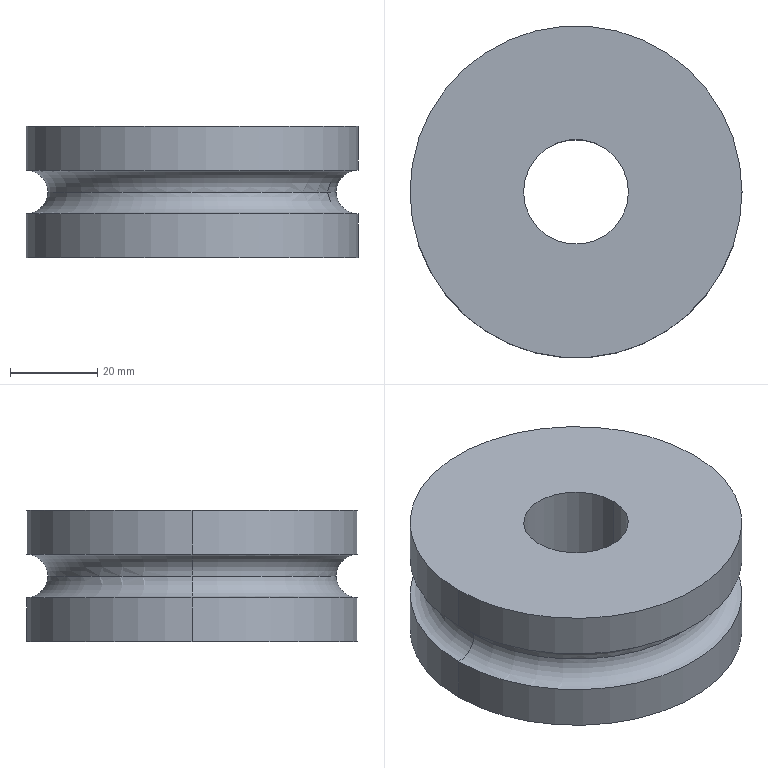Part | SolidWorks | features Extrusion 1, RevCut 1 | 1 solid | 12 faces | box 76 x 76 x 30 mm | volume 113670 mm3 | cylinder 6 | torus 4 | plane 2 | commonest cylinder face diameters 76 x4 24 x2
STEP:
#1=CARTESIAN_POINT('',(-38.,0.,10.));
#2=VERTEX_POINT('',#1);
#3=CARTESIAN_POINT('',(-33.,0.,15.));
#4=VERTEX_POINT('',#3);
#5=CARTESIAN_POINT('',(-38.,0.,15.));
#6=DIRECTION('',(0.,-1.,0.));
#7=DIRECTION('',(0.,0.,-1.));
#8=AXIS2_PLACEMENT_3D('',#5,#6,#7);
#9=CIRCLE('',#8,5.);
#10=EDGE_CURVE('',#2,#4,#9,.T.);
#11=ORIENTED_EDGE('',*,*,#10,.T.);
#12=CARTESIAN_POINT('',(33.,0.,15.));
#13=VERTEX_POINT('',#12);
#14=CARTESIAN_POINT('',(0.,0.,15.));
#15=DIRECTION('',(0.,0.,-1.));
#16=DIRECTION('',(-1.,0.,0.));
#17=AXIS2_PLACEMENT_3D('',#14,#15,#16);
#18=CIRCLE('',#17,33.);
#19=EDGE_CURVE('',#4,#13,#18,.T.);
#20=ORIENTED_EDGE('',*,*,#19,.T.);
#21=CARTESIAN_POINT('',(38.,0.,10.));
#22=VERTEX_POINT('',#21);
#23=CARTESIAN_POINT('',(38.,0.,15.));
#24=DIRECTION('',(0.,1.,0.));
#25=DIRECTION('',(-1.,0.,0.));
#26=AXIS2_PLACEMENT_3D('',#23,#24,#25);
#27=CIRCLE('',#26,5.);
#28=EDGE_CURVE('',#22,#13,#27,.T.);
#29=ORIENTED_EDGE('',*,*,#28,.F.);
#30=CARTESIAN_POINT('',(0.,0.,10.));
#31=DIRECTION('',(0.,0.,-1.));
#32=DIRECTION('',(1.,0.,0.));
#33=AXIS2_PLACEMENT_3D('',#30,#31,#32);
#34=CIRCLE('',#33,38.);
#35=EDGE_CURVE('',#2,#22,#34,.T.);
#36=ORIENTED_EDGE('',*,*,#35,.F.);
#37=EDGE_LOOP('',(#11,#20,#29,#36));
#38=FACE_OUTER_BOUND('',#37,.T.);
#39=CARTESIAN_POINT('',(0.,0.,15.));
#40=DIRECTION('',(0.,0.,-1.));
#41=DIRECTION('',(-1.,0.,0.));
#42=AXIS2_PLACEMENT_3D('',#39,#40,#41);
#43=TOROIDAL_SURFACE('',#42,38.,5.);
#44=ADVANCED_FACE('',(#38),#43,.F.);
#45=ORIENTED_EDGE('',*,*,#28,.T.);
#46=CARTESIAN_POINT('',(0.,0.,15.));
#47=DIRECTION('',(0.,0.,-1.));
#48=DIRECTION('',(-1.,0.,0.));
#49=AXIS2_PLACEMENT_3D('',#46,#47,#48);
#50=CIRCLE('',#49,33.);
#51=EDGE_CURVE('',#13,#4,#50,.T.);
#52=ORIENTED_EDGE('',*,*,#51,.T.);
#53=ORIENTED_EDGE('',*,*,#10,.F.);
#54=CARTESIAN_POINT('',(0.,0.,10.));
#55=DIRECTION('',(0.,0.,-1.));
#56=DIRECTION('',(1.,0.,0.));
#57=AXIS2_PLACEMENT_3D('',#54,#55,#56);
#58=CIRCLE('',#57,38.);
#59=EDGE_CURVE('',#22,#2,#58,.T.);
#60=ORIENTED_EDGE('',*,*,#59,.F.);
#61=EDGE_LOOP('',(#45,#52,#53,#60));
#62=FACE_OUTER_BOUND('',#61,.T.);
#63=CARTESIAN_POINT('',(0.,0.,15.));
#64=DIRECTION('',(0.,0.,-1.));
#65=DIRECTION('',(-1.,0.,0.));
#66=AXIS2_PLACEMENT_3D('',#63,#64,#65);
#67=TOROIDAL_SURFACE('',#66,38.,5.);
#68=ADVANCED_FACE('',(#62),#67,.F.);
#69=ORIENTED_EDGE('',*,*,#51,.F.);
#70=CARTESIAN_POINT('',(38.,0.,20.));
#71=VERTEX_POINT('',#70);
#72=CARTESIAN_POINT('',(38.,0.,15.));
#73=DIRECTION('',(0.,1.,0.));
#74=DIRECTION('',(-1.,0.,0.));
#75=AXIS2_PLACEMENT_3D('',#72,#73,#74);
#76=CIRCLE('',#75,5.);
#77=EDGE_CURVE('',#13,#71,#76,.T.);
#78=ORIENTED_EDGE('',*,*,#77,.T.);
#79=CARTESIAN_POINT('',(-38.,0.,20.));
#80=VERTEX_POINT('',#79);
#81=CARTESIAN_POINT('',(0.,0.,20.));
#82=DIRECTION('',(0.,0.,1.));
#83=DIRECTION('',(-1.,0.,0.));
#84=AXIS2_PLACEMENT_3D('',#81,#82,#83);
#85=CIRCLE('',#84,38.);
#86=EDGE_CURVE('',#80,#71,#85,.T.);
#87=ORIENTED_EDGE('',*,*,#86,.F.);
#88=CARTESIAN_POINT('',(-38.,0.,15.));
#89=DIRECTION('',(0.,-1.,0.));
#90=DIRECTION('',(0.,0.,-1.));
#91=AXIS2_PLACEMENT_3D('',#88,#89,#90);
#92=CIRCLE('',#91,5.);
#93=EDGE_CURVE('',#4,#80,#92,.T.);
#94=ORIENTED_EDGE('',*,*,#93,.F.);
#95=EDGE_LOOP('',(#69,#78,#87,#94));
#96=FACE_OUTER_BOUND('',#95,.T.);
#97=CARTESIAN_POINT('',(0.,0.,15.));
#98=DIRECTION('',(0.,0.,-1.));
#99=DIRECTION('',(-1.,0.,0.));
#100=AXIS2_PLACEMENT_3D('',#97,#98,#99);
#101=TOROIDAL_SURFACE('',#100,38.,5.);
#102=ADVANCED_FACE('',(#96),#101,.F.);
#103=CARTESIAN_POINT('',(-12.,0.,30.));
#104=VERTEX_POINT('',#103);
#105=CARTESIAN_POINT('',(12.,0.,30.));
#106=VERTEX_POINT('',#105);
#107=CARTESIAN_POINT('',(0.,0.,30.));
#108=DIRECTION('',(0.,0.,1.));
#109=DIRECTION('',(1.,0.,0.));
#110=AXIS2_PLACEMENT_3D('',#107,#108,#109);
#111=CIRCLE('',#110,12.);
#112=EDGE_CURVE('',#104,#106,#111,.T.);
#113=ORIENTED_EDGE('',*,*,#112,.T.);
#114=CARTESIAN_POINT('',(12.,0.,0.));
#115=VERTEX_POINT('',#114);
#116=CARTESIAN_POINT('',(12.,0.,30.));
#117=DIRECTION('',(0.,0.,-1.));
#118=VECTOR('',#117,1000.);
#119=LINE('',#116,#118);
#120=EDGE_CURVE('',#106,#115,#119,.T.);
#121=ORIENTED_EDGE('',*,*,#120,.T.);
#122=CARTESIAN_POINT('',(-12.,0.,0.));
#123=VERTEX_POINT('',#122);
#124=CARTESIAN_POINT('',(0.,0.,0.));
#125=DIRECTION('',(0.,0.,1.));
#126=DIRECTION('',(1.,0.,0.));
#127=AXIS2_PLACEMENT_3D('',#124,#125,#126);
#128=CIRCLE('',#127,12.);
#129=EDGE_CURVE('',#123,#115,#128,.T.);
#130=ORIENTED_EDGE('',*,*,#129,.F.);
#131=CARTESIAN_POINT('',(-12.,0.,30.));
#132=DIRECTION('',(0.,0.,-1.));
#133=VECTOR('',#132,1000.);
#134=LINE('',#131,#133);
#135=EDGE_CURVE('',#104,#123,#134,.T.);
#136=ORIENTED_EDGE('',*,*,#135,.F.);
#137=EDGE_LOOP('',(#113,#121,#130,#136));
#138=FACE_OUTER_BOUND('',#137,.T.);
#139=CARTESIAN_POINT('',(0.,0.,30.));
#140=DIRECTION('',(0.,0.,-1.));
#141=DIRECTION('',(-1.,0.,0.));
#142=AXIS2_PLACEMENT_3D('',#139,#140,#141);
#143=CYLINDRICAL_SURFACE('',#142,12.);
#144=ADVANCED_FACE('',(#138),#143,.F.);
#145=CARTESIAN_POINT('',(38.,0.,30.));
#146=VERTEX_POINT('',#145);
#147=CARTESIAN_POINT('',(-38.,0.,30.));
#148=VERTEX_POINT('',#147);
#149=CARTESIAN_POINT('',(0.,0.,30.));
#150=DIRECTION('',(0.,0.,1.));
#151=DIRECTION('',(1.,0.,0.));
#152=AXIS2_PLACEMENT_3D('',#149,#150,#151);
#153=CIRCLE('',#152,38.);
#154=EDGE_CURVE('',#146,#148,#153,.T.);
#155=ORIENTED_EDGE('',*,*,#154,.F.);
#156=CARTESIAN_POINT('',(38.,0.,30.));
#157=DIRECTION('',(0.,0.,-1.));
#158=VECTOR('',#157,1000.);
#159=LINE('',#156,#158);
#160=EDGE_CURVE('',#146,#71,#159,.T.);
#161=ORIENTED_EDGE('',*,*,#160,.T.);
#162=CARTESIAN_POINT('',(0.,0.,20.));
#163=DIRECTION('',(0.,0.,1.));
#164=DIRECTION('',(-1.,0.,0.));
#165=AXIS2_PLACEMENT_3D('',#162,#163,#164);
#166=CIRCLE('',#165,38.);
#167=EDGE_CURVE('',#71,#80,#166,.T.);
#168=ORIENTED_EDGE('',*,*,#167,.T.);
#169=CARTESIAN_POINT('',(-38.,0.,30.));
#170=DIRECTION('',(0.,0.,-1.));
#171=VECTOR('',#170,1000.);
#172=LINE('',#169,#171);
#173=EDGE_CURVE('',#148,#80,#172,.T.);
#174=ORIENTED_EDGE('',*,*,#173,.F.);
#175=EDGE_LOOP('',(#155,#161,#168,#174));
#176=FACE_OUTER_BOUND('',#175,.T.);
#177=CARTESIAN_POINT('',(0.,0.,30.));
#178=DIRECTION('',(0.,0.,-1.));
#179=DIRECTION('',(-1.,0.,0.));
#180=AXIS2_PLACEMENT_3D('',#177,#178,#179);
#181=CYLINDRICAL_SURFACE('',#180,38.);
#182=ADVANCED_FACE('',(#176),#181,.T.);
#183=ORIENTED_EDGE('',*,*,#35,.T.);
#184=CARTESIAN_POINT('',(38.,0.,0.));
#185=VERTEX_POINT('',#184);
#186=CARTESIAN_POINT('',(38.,0.,30.));
#187=DIRECTION('',(0.,0.,-1.));
#188=VECTOR('',#187,1000.);
#189=LINE('',#186,#188);
#190=EDGE_CURVE('',#22,#185,#189,.T.);
#191=ORIENTED_EDGE('',*,*,#190,.T.);
#192=CARTESIAN_POINT('',(-38.,0.,0.));
#193=VERTEX_POINT('',#192);
#194=CARTESIAN_POINT('',(0.,0.,0.));
#195=DIRECTION('',(0.,0.,1.));
#196=DIRECTION('',(1.,0.,0.));
#197=AXIS2_PLACEMENT_3D('',#194,#195,#196);
#198=CIRCLE('',#197,38.);
#199=EDGE_CURVE('',#185,#193,#198,.T.);
#200=ORIENTED_EDGE('',*,*,#199,.T.);
#201=CARTESIAN_POINT('',(-38.,0.,30.));
#202=DIRECTION('',(0.,0.,-1.));
#203=VECTOR('',#202,1000.);
#204=LINE('',#201,#203);
#205=EDGE_CURVE('',#2,#193,#204,.T.);
#206=ORIENTED_EDGE('',*,*,#205,.F.);
#207=EDGE_LOOP('',(#183,#191,#200,#206));
#208=FACE_OUTER_BOUND('',#207,.T.);
#209=CARTESIAN_POINT('',(0.,0.,30.));
#210=DIRECTION('',(0.,0.,-1.));
#211=DIRECTION('',(-1.,0.,0.));
#212=AXIS2_PLACEMENT_3D('',#209,#210,#211);
#213=CYLINDRICAL_SURFACE('',#212,38.);
#214=ADVANCED_FACE('',(#208),#213,.T.);
#215=ORIENTED_EDGE('',*,*,#190,.F.);
#216=ORIENTED_EDGE('',*,*,#59,.T.);
#217=ORIENTED_EDGE('',*,*,#205,.T.);
#218=CARTESIAN_POINT('',(0.,0.,0.));
#219=DIRECTION('',(0.,0.,1.));
#220=DIRECTION('',(1.,0.,0.));
#221=AXIS2_PLACEMENT_3D('',#218,#219,#220);
#222=CIRCLE('',#221,38.);
#223=EDGE_CURVE('',#193,#185,#222,.T.);
#224=ORIENTED_EDGE('',*,*,#223,.T.);
#225=EDGE_LOOP('',(#215,#216,#217,#224));
#226=FACE_OUTER_BOUND('',#225,.T.);
#227=CARTESIAN_POINT('',(0.,0.,30.));
#228=DIRECTION('',(0.,0.,-1.));
#229=DIRECTION('',(-1.,0.,0.));
#230=AXIS2_PLACEMENT_3D('',#227,#228,#229);
#231=CYLINDRICAL_SURFACE('',#230,38.);
#232=ADVANCED_FACE('',(#226),#231,.T.);
#233=CARTESIAN_POINT('',(0.,0.,30.));
#234=DIRECTION('',(0.,0.,1.));
#235=DIRECTION('',(1.,0.,0.));
#236=AXIS2_PLACEMENT_3D('',#233,#234,#235);
#237=CIRCLE('',#236,38.);
#238=EDGE_CURVE('',#148,#146,#237,.T.);
#239=ORIENTED_EDGE('',*,*,#238,.T.);
#240=ORIENTED_EDGE('',*,*,#154,.T.);
#241=EDGE_LOOP('',(#239,#240));
#242=FACE_OUTER_BOUND('',#241,.T.);
#243=ORIENTED_EDGE('',*,*,#112,.F.);
#244=CARTESIAN_POINT('',(0.,0.,30.));
#245=DIRECTION('',(0.,0.,1.));
#246=DIRECTION('',(1.,0.,0.));
#247=AXIS2_PLACEMENT_3D('',#244,#245,#246);
#248=CIRCLE('',#247,12.);
#249=EDGE_CURVE('',#106,#104,#248,.T.);
#250=ORIENTED_EDGE('',*,*,#249,.F.);
#251=EDGE_LOOP('',(#243,#250));
#252=FACE_BOUND('',#251,.T.);
#253=CARTESIAN_POINT('',(0.,0.,30.));
#254=DIRECTION('',(0.,0.,1.));
#255=DIRECTION('',(1.,0.,0.));
#256=AXIS2_PLACEMENT_3D('',#253,#254,#255);
#257=PLANE('',#256);
#258=ADVANCED_FACE('',(#242,#252),#257,.T.);
#259=ORIENTED_EDGE('',*,*,#223,.F.);
#260=ORIENTED_EDGE('',*,*,#199,.F.);
#261=EDGE_LOOP('',(#259,#260));
#262=FACE_OUTER_BOUND('',#261,.T.);
#263=ORIENTED_EDGE('',*,*,#129,.T.);
#264=CARTESIAN_POINT('',(0.,0.,0.));
#265=DIRECTION('',(0.,0.,1.));
#266=DIRECTION('',(1.,0.,0.));
#267=AXIS2_PLACEMENT_3D('',#264,#265,#266);
#268=CIRCLE('',#267,12.);
#269=EDGE_CURVE('',#115,#123,#268,.T.);
#270=ORIENTED_EDGE('',*,*,#269,.T.);
#271=EDGE_LOOP('',(#263,#270));
#272=FACE_BOUND('',#271,.T.);
#273=CARTESIAN_POINT('',(0.,0.,0.));
#274=DIRECTION('',(0.,0.,1.));
#275=DIRECTION('',(1.,0.,0.));
#276=AXIS2_PLACEMENT_3D('',#273,#274,#275);
#277=PLANE('',#276);
#278=ADVANCED_FACE('',(#262,#272),#277,.F.);
#279=ORIENTED_EDGE('',*,*,#160,.F.);
#280=ORIENTED_EDGE('',*,*,#238,.F.);
#281=ORIENTED_EDGE('',*,*,#173,.T.);
#282=ORIENTED_EDGE('',*,*,#86,.T.);
#283=EDGE_LOOP('',(#279,#280,#281,#282));
#284=FACE_OUTER_BOUND('',#283,.T.);
#285=CARTESIAN_POINT('',(0.,0.,30.));
#286=DIRECTION('',(0.,0.,-1.));
#287=DIRECTION('',(-1.,0.,0.));
#288=AXIS2_PLACEMENT_3D('',#285,#286,#287);
#289=CYLINDRICAL_SURFACE('',#288,38.);
#290=ADVANCED_FACE('',(#284),#289,.T.);
#291=ORIENTED_EDGE('',*,*,#120,.F.);
#292=ORIENTED_EDGE('',*,*,#249,.T.);
#293=ORIENTED_EDGE('',*,*,#135,.T.);
#294=ORIENTED_EDGE('',*,*,#269,.F.);
#295=EDGE_LOOP('',(#291,#292,#293,#294));
#296=FACE_OUTER_BOUND('',#295,.T.);
#297=CARTESIAN_POINT('',(0.,0.,30.));
#298=DIRECTION('',(0.,0.,-1.));
#299=DIRECTION('',(-1.,0.,0.));
#300=AXIS2_PLACEMENT_3D('',#297,#298,#299);
#301=CYLINDRICAL_SURFACE('',#300,12.);
#302=ADVANCED_FACE('',(#296),#301,.F.);
#303=ORIENTED_EDGE('',*,*,#19,.F.);
#304=ORIENTED_EDGE('',*,*,#93,.T.);
#305=ORIENTED_EDGE('',*,*,#167,.F.);
#306=ORIENTED_EDGE('',*,*,#77,.F.);
#307=EDGE_LOOP('',(#303,#304,#305,#306));
#308=FACE_OUTER_BOUND('',#307,.T.);
#309=CARTESIAN_POINT('',(0.,0.,15.));
#310=DIRECTION('',(0.,0.,-1.));
#311=DIRECTION('',(-1.,0.,0.));
#312=AXIS2_PLACEMENT_3D('',#309,#310,#311);
#313=TOROIDAL_SURFACE('',#312,38.,5.);
#314=ADVANCED_FACE('',(#308),#313,.F.);
#315=CLOSED_SHELL('',(#44,#68,#102,#144,#182,#214,#232,#258,#278,#290,#302,#314));
#316=MANIFOLD_SOLID_BREP('',#315);
#317=CARTESIAN_POINT('',(0.,0.,0.));
#318=DIRECTION('',(0.,0.,1.));
#319=DIRECTION('',(1.,0.,0.));
#320=AXIS2_PLACEMENT_3D('',#317,#318,#319);
#321=(LENGTH_UNIT()NAMED_UNIT(*)SI_UNIT(.MILLI.,.METRE.));
#322=UNCERTAINTY_MEASURE_WITH_UNIT(LENGTH_MEASURE(0.00001),#321,'','');
#323=(NAMED_UNIT(*)PLANE_ANGLE_UNIT()SI_UNIT($,.RADIAN.));
#324=(NAMED_UNIT(*)SI_UNIT($,.STERADIAN.)SOLID_ANGLE_UNIT());
#325=(GEOMETRIC_REPRESENTATION_CONTEXT(3)GLOBAL_UNCERTAINTY_ASSIGNED_CONTEXT((#322))GLOBAL_UNIT_ASSIGNED_CONTEXT((#321,#323,#324))REPRESENTATION_CONTEXT('',''));
#326=ADVANCED_BREP_SHAPE_REPRESENTATION('',(#316,#320),#325);